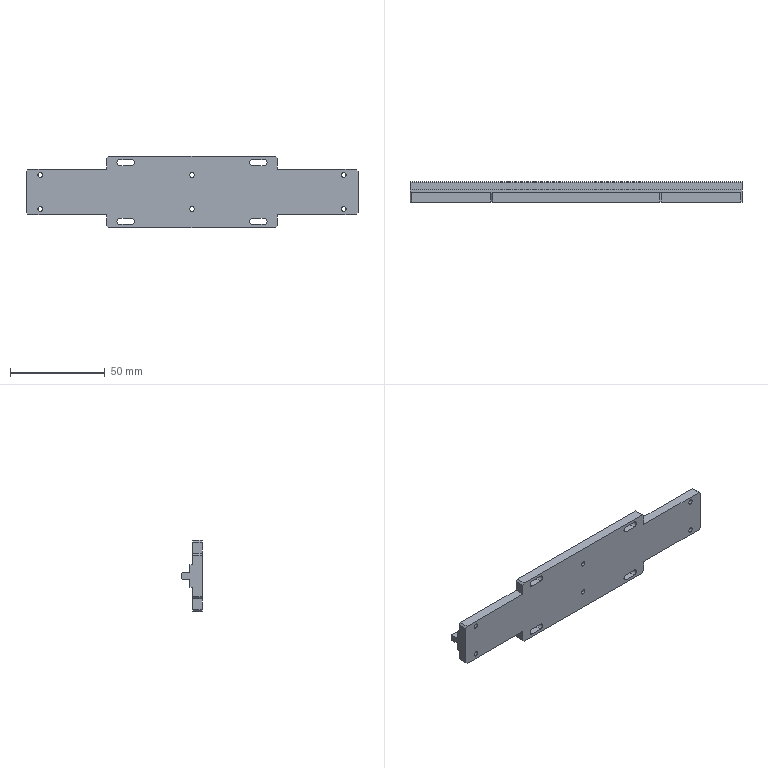Part | STEP file | PN_0018 | 1 solid | 60 faces | box 175 x 10.7 x 37.5 mm | volume 32070 mm3 | plane 40 | cylinder 20 | commonest cylinder face diameters 2.5 x12 3.2 x8